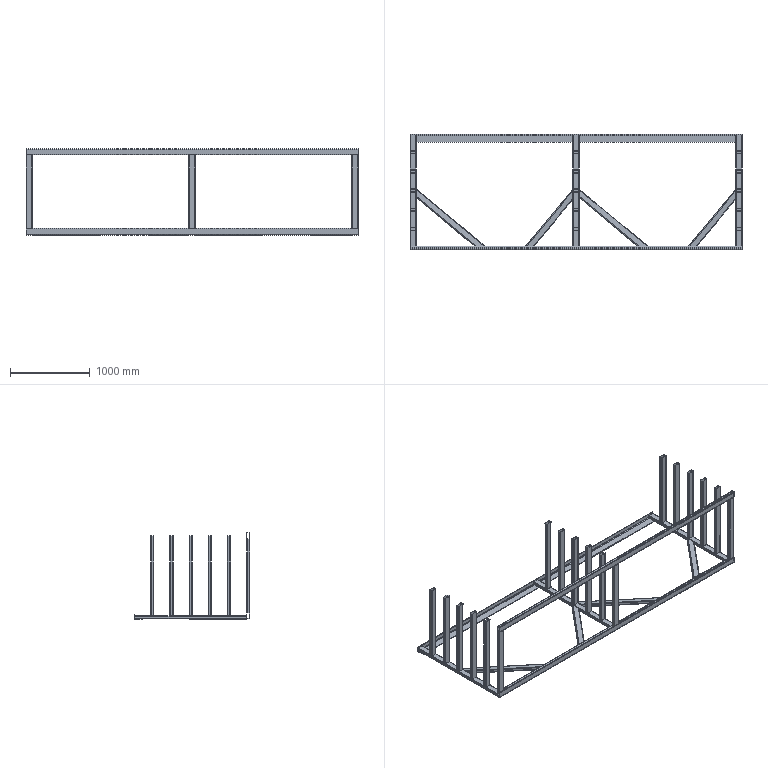Part | SolidWorks | features WeldCornerFeat 7, 3DProfileFeature 2, MoveCopyBody 2, WeldMemberFeat 2, WeldmentFeature 1 | 28 solids | 507 faces | box 4160 x 1446 x 1089 mm | volume 33111474 mm3 | plane 280 | cylinder 227 | commonest cylinder face diameters 8 x112 16 x112 4 x2 20 x1